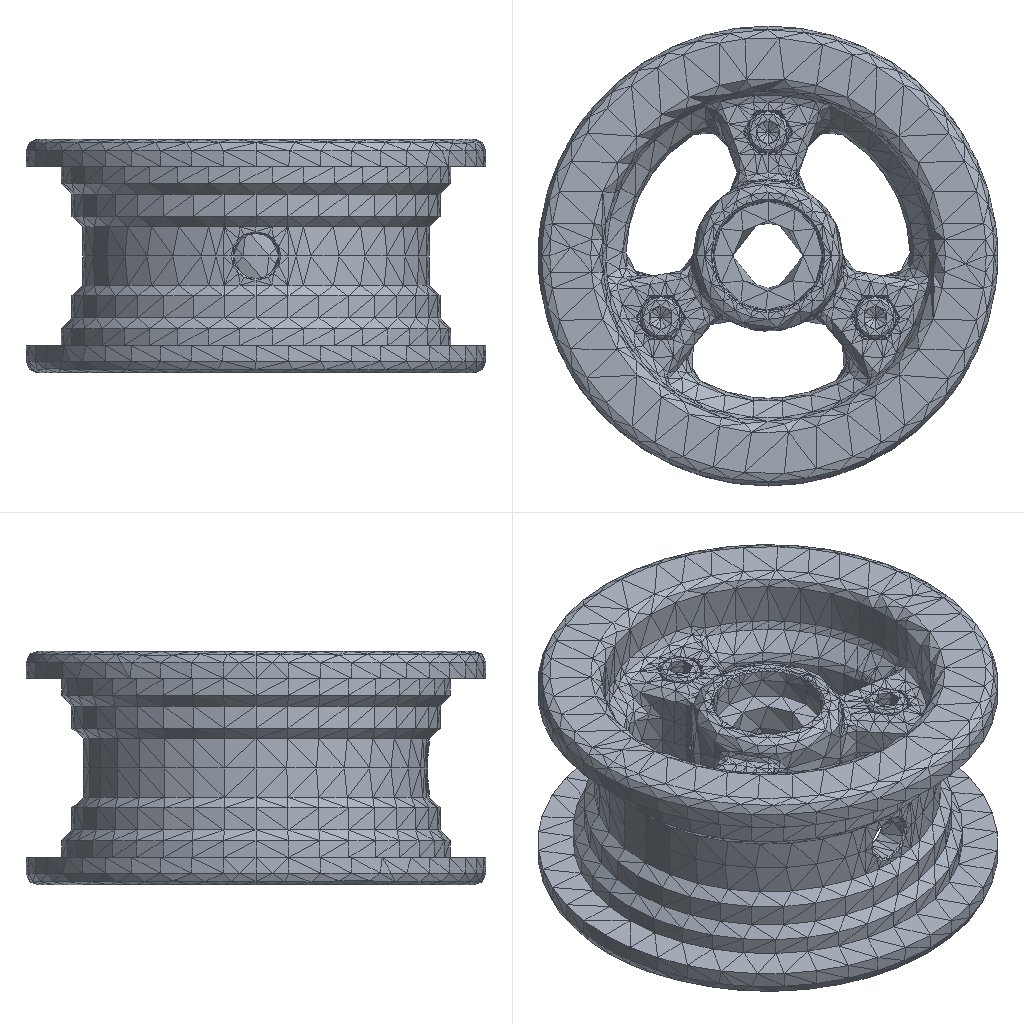Simulation study | ansys workbench
Ansys APDL input file, long lists of numbers shortened:
/batch
/config,noeldb,1     ! force off writing results to database
*get,_wallstrt,active,,time,wall
! ANSYS input file written by Workbench version 2022 R1
! File used for geometry attach:
/title,wbnew--____ (D5)
! ****** Begin Custom Load Command Snippet ******
/COM, ACT Extensions:
/COM,     LSDYNA, 2021.1
/COM,
! ****** End   Custom Load Command Snippet ******
*DIM,_wb_ProjectScratch_dir,string,248
_wb_ProjectScratch_dir(1) = ''
*DIM,_wb_SolverFiles_dir,string,248
_wb_SolverFiles_dir(1) = ''
*DIM,_wb_userfiles_dir,string,248
_wb_userfiles_dir(1) = ''
/com,--- Data in consistent NMM units. See Solving Units in the help system for more information.
/units,MPA
/nopr
/wb,file,start              !  signify a WB generated input file
/prep7
! Turn off shape checking because checks already performed inside WB mesher.
! See help system for more information.
SHPP,OFF,,NOWARN
/nolist
etcon,set             ! allow ANSYS to choose best KEYOP's for 180x elements, resets any applicable keyopt to MAPDL defaults
/com,*********** Nodes for the whole assembly ***********
nblock,3,,38121
(1i9,3e20.9e3)
        1    -5.164900630E+01     4.284439535E+01     3.826096569E+01
! (34655 more lines like these left out)
-1
/com,*********** Nodes for all Remote Points ***********
nblock,3
(1i9,3e20.9e3)
    34657    -5.164900630E+01     1.223253645E+01     3.003884414E+01
-1
/wb,elem,start            !  set before creation of elements
/com,*********** Elements for Body 1 "Wheel Hub|Pah4" ***********
et,1,187
eblock,19,solid,,6596
(19i9)
        1        1        1        1        0        0        0        0       10        0    11937    23119    23893    24445    24099    29033    33173    29038    29035
! (13191 more lines like these left out)
-1
/com,*********** Elements for Body 2 "Wheel Hub|Pah4[2]" ***********
et,2,187
eblock,19,solid,,6596
(19i9)
        2        2        2        2        0        0        0        0       10        0     5341    10933    11707    12259    11913    16847    20987    16852    16849
! (13191 more lines like these left out)
-1
/com,*********** Elements for Body 3 "socket head cap screw_am32323_PreviewCfg|____1" ***********
et,3,187
eblock,19,solid,,671
(19i9)
        3        3        3        3        0        0        0        0       10        0      672     1298     1415     1505     1489     1616     2262     1622     1620
! (1341 more lines like these left out)
-1
/com,*********** Elements for Body 4 "socket head cap screw_am32323_PreviewCfg|____1[2]" ***********
et,4,187
eblock,19,solid,,671
(19i9)
        4        4        4        4        0        0        0        0       10        0     3561     6868     6985     7075     7059     7186     7832     7192     7190
! (1341 more lines like these left out)
-1
/com,*********** Elements for Body 5 "socket head cap screw_am32323_PreviewCfg|____1[3]" ***********
et,5,187
eblock,19,solid,,671
(19i9)
        5        5        5        5        0        0        0        0       10        0        1       12      129      219      203      330      976      336      334
! (1341 more lines like these left out)
-1
/com,*********** Elements for Body 6 "hex nut style 1_am333_PreviewCfg|____1" ***********
et,6,187
eblock,19,solid,,1109
(19i9)
        6        6        6        6        0        0        0        0       10        0     2452     5022     5083     5045     5077     6728     6812     6724     6726
! (2217 more lines like these left out)
-1
/com,*********** Elements for Body 7 "hex nut style 1_am333_PreviewCfg|____1[2]" ***********
et,7,187
eblock,19,solid,,1109
(19i9)
        7        7        7        7        0        0        0        0       10        0     4232     8450     8511     8473     8505    10156    10240    10152    10154
! (2217 more lines like these left out)
-1
/com,*********** Elements for Body 8 "hex nut style 1_am333_PreviewCfg|____1[3]" ***********
et,8,187
eblock,19,solid,,1109
(19i9)
        8        8        8        8        0        0        0        0       10        0     1343     2880     2941     2903     2935     4586     4670     4582     4584
! (2217 more lines like these left out)
-1
/wb,elem,end               !  done creating elements
/com,*********** Send User Defined Coordinate System(s) ***********
csys,0
toffst,273.15,  ! Temperature offset from absolute zero
/com,*********** Set Reference Temperature ***********
tref,22.
/wb,mat,start              !  starting to send materials
/com,*********** Send Materials ***********
Temperature = 'TEMP' ! Temperature
MP,DENS,1,7.85e-09,	! tonne mm^-3
MP,ALPX,1,1.2e-05,	! C^-1
MP,C,1,434000000,	! mm^2 s^-2 C^-1
MP,KXX,1,60.5,	! tonne mm s^-3 C^-1
MP,RSVX,1,0.00017,	! ohm mm
MP,EX,1,200000,	! tonne s^-2 mm^-1
MP,NUXY,1,0.3,
MP,MURX,1,10000,
Temperature = 'TEMP' ! Temperature
MP,DENS,2,7.85e-09,	! tonne mm^-3
MP,ALPX,2,1.2e-05,	! C^-1
MP,C,2,434000000,	! mm^2 s^-2 C^-1
MP,KXX,2,60.5,	! tonne mm s^-3 C^-1
MP,RSVX,2,0.00017,	! ohm mm
MP,EX,2,200000,	! tonne s^-2 mm^-1
MP,NUXY,2,0.3,
MP,MURX,2,10000,
Temperature = 'TEMP' ! Temperature
MP,DENS,3,7.85e-09,	! tonne mm^-3
MP,ALPX,3,1.2e-05,	! C^-1
MP,C,3,434000000,	! mm^2 s^-2 C^-1
MP,KXX,3,60.5,	! tonne mm s^-3 C^-1
MP,RSVX,3,0.00017,	! ohm mm
MP,EX,3,200000,	! tonne s^-2 mm^-1
MP,NUXY,3,0.3,
MP,MURX,3,10000,
Temperature = 'TEMP' ! Temperature
MP,DENS,4,7.85e-09,	! tonne mm^-3
MP,ALPX,4,1.2e-05,	! C^-1
MP,C,4,434000000,	! mm^2 s^-2 C^-1
MP,KXX,4,60.5,	! tonne mm s^-3 C^-1
MP,RSVX,4,0.00017,	! ohm mm
MP,EX,4,200000,	! tonne s^-2 mm^-1
MP,NUXY,4,0.3,
MP,MURX,4,10000,
Temperature = 'TEMP' ! Temperature
MP,DENS,5,7.85e-09,	! tonne mm^-3
MP,ALPX,5,1.2e-05,	! C^-1
MP,C,5,434000000,	! mm^2 s^-2 C^-1
MP,KXX,5,60.5,	! tonne mm s^-3 C^-1
MP,RSVX,5,0.00017,	! ohm mm
MP,EX,5,200000,	! tonne s^-2 mm^-1
MP,NUXY,5,0.3,
MP,MURX,5,10000,
Temperature = 'TEMP' ! Temperature
MP,DENS,6,7.85e-09,	! tonne mm^-3
MP,ALPX,6,1.2e-05,	! C^-1
MP,C,6,434000000,	! mm^2 s^-2 C^-1
MP,KXX,6,60.5,	! tonne mm s^-3 C^-1
MP,RSVX,6,0.00017,	! ohm mm
MP,EX,6,200000,	! tonne s^-2 mm^-1
MP,NUXY,6,0.3,
MP,MURX,6,10000,
Temperature = 'TEMP' ! Temperature
MP,DENS,7,7.85e-09,	! tonne mm^-3
MP,ALPX,7,1.2e-05,	! C^-1
MP,C,7,434000000,	! mm^2 s^-2 C^-1
MP,KXX,7,60.5,	! tonne mm s^-3 C^-1
MP,RSVX,7,0.00017,	! ohm mm
MP,EX,7,200000,	! tonne s^-2 mm^-1
MP,NUXY,7,0.3,
MP,MURX,7,10000,
Temperature = 'TEMP' ! Temperature
MP,DENS,8,7.85e-09,	! tonne mm^-3
MP,ALPX,8,1.2e-05,	! C^-1
MP,C,8,434000000,	! mm^2 s^-2 C^-1
MP,KXX,8,60.5,	! tonne mm s^-3 C^-1
MP,RSVX,8,0.00017,	! ohm mm
MP,EX,8,200000,	! tonne s^-2 mm^-1
MP,NUXY,8,0.3,
MP,MURX,8,10000,
/wb,mat,end                !  done sending materials
!************************* Model Summary ********************
!Wheel Hub|Pah4,	6061,	matid,	1
!Wheel Hub|Pah4[2],	6061,	matid,	2
!socket head cap screw_am32323_PreviewCfg|____1,	6061,	matid,	3
!socket head cap screw_am32323_PreviewCfg|____1[2],	6061,	matid,	4
!socket head cap screw_am32323_PreviewCfg|____1[3],	6061,	matid,	5
!hex nut style 1_am333_PreviewCfg|____1,	6061,	matid,	6
!hex nut style 1_am333_PreviewCfg|____1[2],	6061,	matid,	7
!hex nut style 1_am333_PreviewCfg|____1[3],	6061,	matid,	8
!************************* End Model Summary ********************
! get the diagonal of the bounding box. Needed later for other things
*get,_xmin,node,,mnloc,x
*get,_ymin,node,,mnloc,y
*get,_zmin,node,,mnloc,z
*get,_xmax,node,,mxloc,x
*get,_ymax,node,,mxloc,y
*get,_zmax,node,,mxloc,z
_ASMDIAG=(_xmax-_xmin)*(_xmax-_xmin)+(_ymax-_ymin)*(_ymax-_ymin)+(_zmax-_zmin)*(_zmax-_zmin)
_ASMDIAG=SQRT(_ASMDIAG)
/wb,contact,start          !  starting to send contact
/com,*********** Create Contact "接触区域" ***********
/com,            Real Constant Set For Above Contact Is 10 & 9
*set,tid,10
*set,cid,9
r,tid
r,cid
et,tid,170
et,cid,174
eblock,10,,,292
(15i9)
    27844       10       10       10        0    22495    22497    22499    22499    24605    24622    22499    24606
! (291 more lines like these left out)
-1
eblock,10,,,292
(15i9)
    28136        9        9        9        0    22495    22497    22499    22499    24605    24622    22499    24606
! (291 more lines like these left out)
-1
eblock,10,,,292
(15i9)
    28428        9       10        9        0    10324    10794    11362    11362    12531    15894    11362    12532
! (291 more lines like these left out)
-1
eblock,10,,,292
(15i9)
    28720       10        9       10        0    10324    10794    11362    11362    12531    15894    11362    12532
! (291 more lines like these left out)
-1
keyo,cid,8,2               ! auto create asymmetric contact (from Program Controlled setting)
keyo,cid,10,0              ! adjust contact stiffness each NR iteration (from Program Controlled setting)
keyo,cid,12,5              ! bonded always
keyo,cid,18,1              ! small sliding turned on by application
keyo,cid,2,0               ! augmented Lagrange (from Program Controlled setting)
keyo,cid,4,0               ! on Gauss point (from Program Controlled setting)
keyo,cid,9,1               ! ignore initial gaps/penetration
keyo,cid,7,0               ! No Prediction
rmod,tid,3,10.      ! FKN
rmod,tid,5,0.       ! ICONT
rmod,tid,6,0.       ! PINB
rmod,tid,10,0.      ! CNOF
rmod,tid,12,0.      ! FKT
rmod,tid,36,47      ! WB DSID
rmod,cid,3,10.      ! FKN
rmod,cid,5,0.       ! ICONT
rmod,cid,6,0.       ! PINB
rmod,cid,10,0.      ! CNOF
rmod,cid,12,0.      ! FKT
rmod,cid,36,47      ! WB DSID
/com,*********** Create Contact "接触区域 2" ***********
/com,            Real Constant Set For Above Contact Is 12 & 11
*set,tid,12
*set,cid,11
r,tid
r,cid
et,tid,170
et,cid,174
eblock,10,,,78
(15i9)
    29012       12       12       12        0    22918    22919    23454    23454    27724    27731    23454    27725
! (77 more lines like these left out)
-1
eblock,10,,,78
(15i9)
    29090       11       11       11        0    22918    22919    23454    23454    27724    27731    23454    27725
! (77 more lines like these left out)
-1
eblock,10,,,120
(15i9)
    29168       11       12       11        0     1400     1399     1303     1303     2184     1657     1303     1658
! (119 more lines like these left out)
-1
eblock,10,,,120
(15i9)
    29288       12       11       12        0     1400     1399     1303     1303     2184     1657     1303     1658
! (119 more lines like these left out)
-1
keyo,cid,8,2               ! auto create asymmetric contact (from Program Controlled setting)
keyo,cid,10,0              ! adjust contact stiffness each NR iteration (from Program Controlled setting)
keyo,cid,12,5              ! bonded always
keyo,cid,18,1              ! small sliding turned on by application
keyo,cid,2,0               ! augmented Lagrange (from Program Controlled setting)
keyo,cid,4,0               ! on Gauss point (from Program Controlled setting)
keyo,cid,9,1               ! ignore initial gaps/penetration
keyo,cid,7,0               ! No Prediction
rmod,tid,3,10.      ! FKN
rmod,tid,5,0.       ! ICONT
rmod,tid,6,0.       ! PINB
rmod,tid,10,0.      ! CNOF
rmod,tid,12,0.      ! FKT
rmod,tid,36,50      ! WB DSID
rmod,cid,3,10.      ! FKN
rmod,cid,5,0.       ! ICONT
rmod,cid,6,0.       ! PINB
rmod,cid,10,0.      ! CNOF
rmod,cid,12,0.      ! FKT
rmod,cid,36,50      ! WB DSID
/com,*********** Create Contact "接触区域 3" ***********
/com,            Real Constant Set For Above Contact Is 14 & 13
*set,tid,14
*set,cid,13
r,tid
r,cid
et,tid,170
et,cid,174
eblock,10,,,78
(15i9)
    29408       14       14       14        0    22926    23468    23463    23463    27781    31254    23463    27780
! (77 more lines like these left out)
-1
eblock,10,,,78
(15i9)
    29486       13       13       13        0    22926    23468    23463    23463    27781    31254    23463    27780
! (77 more lines like these left out)
-1
eblock,10,,,120
(15i9)
    29564       13       14       13        0     6970     6969     6873     6873     7754     7227     6873     7228
! (119 more lines like these left out)
-1
eblock,10,,,120
(15i9)
    29684       14       13       14        0     6970     6969     6873     6873     7754     7227     6873     7228
! (119 more lines like these left out)
-1
keyo,cid,8,2               ! auto create asymmetric contact (from Program Controlled setting)
keyo,cid,10,0              ! adjust contact stiffness each NR iteration (from Program Controlled setting)
keyo,cid,12,5              ! bonded always
keyo,cid,18,1              ! small sliding turned on by application
keyo,cid,2,0               ! augmented Lagrange (from Program Controlled setting)
keyo,cid,4,0               ! on Gauss point (from Program Controlled setting)
keyo,cid,9,1               ! ignore initial gaps/penetration
keyo,cid,7,0               ! No Prediction
rmod,tid,3,10.      ! FKN
rmod,tid,5,0.       ! ICONT
rmod,tid,6,0.       ! PINB
rmod,tid,10,0.      ! CNOF
rmod,tid,12,0.      ! FKT
rmod,tid,36,53      ! WB DSID
rmod,cid,3,10.      ! FKN
rmod,cid,5,0.       ! ICONT
rmod,cid,6,0.       ! PINB
rmod,cid,10,0.      ! CNOF
rmod,cid,12,0.      ! FKT
rmod,cid,36,53      ! WB DSID
/com,*********** Create Contact "接触区域 4" ***********
/com,            Real Constant Set For Above Contact Is 16 & 15
*set,tid,16
*set,cid,15
r,tid
r,cid
et,tid,170
et,cid,174
eblock,10,,,96
(15i9)
    29804       16       16       16        0    22908    23705    23140    23140    27661    29200    23140    27658
! (95 more lines like these left out)
-1
eblock,10,,,96
(15i9)
    29900       15       15       15        0    22908    23705    23140    23140    27661    29200    23140    27658
! (95 more lines like these left out)
-1
eblock,10,,,120
(15i9)
    29996       15       16       15        0      114      113       17       17      898      371       17      372
! (119 more lines like these left out)
-1
eblock,10,,,120
(15i9)
    30116       16       15       16        0      114      113       17       17      898      371       17      372
! (119 more lines like these left out)
-1
keyo,cid,8,2               ! auto create asymmetric contact (from Program Controlled setting)
keyo,cid,10,0              ! adjust contact stiffness each NR iteration (from Program Controlled setting)
keyo,cid,12,5              ! bonded always
keyo,cid,18,1              ! small sliding turned on by application
keyo,cid,2,0               ! augmented Lagrange (from Program Controlled setting)
keyo,cid,4,0               ! on Gauss point (from Program Controlled setting)
keyo,cid,9,1               ! ignore initial gaps/penetration
keyo,cid,7,0               ! No Prediction
rmod,tid,3,10.      ! FKN
rmod,tid,5,0.       ! ICONT
rmod,tid,6,0.       ! PINB
rmod,tid,10,0.      ! CNOF
rmod,tid,12,0.      ! FKT
rmod,tid,36,56      ! WB DSID
rmod,cid,3,10.      ! FKN
rmod,cid,5,0.       ! ICONT
rmod,cid,6,0.       ! PINB
rmod,cid,10,0.      ! CNOF
rmod,cid,12,0.      ! FKT
rmod,cid,36,56      ! WB DSID
/com,*********** Create Contact "接触区域 5" ***********
/com,            Real Constant Set For Above Contact Is 18 & 17
*set,tid,18
*set,cid,17
r,tid
r,cid
et,tid,170
et,cid,174
eblock,10,,,12
(15i9)
    30236       18       18       18        0    10732    10733    11268    11268    15538    15545    11268    15539
! (11 more lines like these left out)
-1
eblock,10,,,12
(15i9)
    30248       17       17       17        0    10732    10733    11268    11268    15538    15545    11268    15539
! (11 more lines like these left out)
-1
eblock,10,,,154
(15i9)
    30260       17       18       17        0     4879     4937     4987     4987     6115     6303     4987     6117
! (153 more lines like these left out)
-1
eblock,10,,,154
(15i9)
    30414       18       17       18        0     4879     4937     4987     4987     6115     6303     4987     6117
! (153 more lines like these left out)
-1
keyo,cid,8,2               ! auto create asymmetric contact (from Program Controlled setting)
keyo,cid,10,0              ! adjust contact stiffness each NR iteration (from Program Controlled setting)
keyo,cid,12,5              ! bonded always
keyo,cid,18,1              ! small sliding turned on by application
keyo,cid,2,0               ! augmented Lagrange (from Program Controlled setting)
keyo,cid,4,0               ! on Gauss point (from Program Controlled setting)
keyo,cid,9,1               ! ignore initial gaps/penetration
keyo,cid,7,0               ! No Prediction
rmod,tid,3,10.      ! FKN
rmod,tid,5,0.       ! ICONT
rmod,tid,6,0.       ! PINB
rmod,tid,10,0.      ! CNOF
rmod,tid,12,0.      ! FKT
rmod,tid,36,59      ! WB DSID
rmod,cid,3,10.      ! FKN
rmod,cid,5,0.       ! ICONT
rmod,cid,6,0.       ! PINB
rmod,cid,10,0.      ! CNOF
rmod,cid,12,0.      ! FKT
rmod,cid,36,59      ! WB DSID
/com,*********** Create Contact "接触区域 6" ***********
/com,            Real Constant Set For Above Contact Is 20 & 19
*set,tid,20
*set,cid,19
r,tid
r,cid
et,tid,170
et,cid,174
eblock,10,,,19
(15i9)
    30568       20       20       20        0    10722    11519    10954    10954    15475    17014    10954    15472
! (18 more lines like these left out)
-1
eblock,10,,,19
(15i9)
    30587       19       19       19        0    10722    11519    10954    10954    15475    17014    10954    15472
! (18 more lines like these left out)
-1
eblock,10,,,147
(15i9)
    30606       19       20       19        0     8307     8365     8415     8415     9543     9731     8415     9545
! (146 more lines like these left out)
-1
eblock,10,,,147
(15i9)
    30753       20       19       20        0     8307     8365     8415     8415     9543     9731     8415     9545
! (146 more lines like these left out)
-1
keyo,cid,8,2               ! auto create asymmetric contact (from Program Controlled setting)
keyo,cid,10,0              ! adjust contact stiffness each NR iteration (from Program Controlled setting)
keyo,cid,12,5              ! bonded always
keyo,cid,18,1              ! small sliding turned on by application
keyo,cid,2,0               ! augmented Lagrange (from Program Controlled setting)
keyo,cid,4,0               ! on Gauss point (from Program Controlled setting)
keyo,cid,9,1               ! ignore initial gaps/penetration
keyo,cid,7,0               ! No Prediction
rmod,tid,3,10.      ! FKN
rmod,tid,5,0.       ! ICONT
rmod,tid,6,0.       ! PINB
rmod,tid,10,0.      ! CNOF
rmod,tid,12,0.      ! FKT
rmod,tid,36,62      ! WB DSID
rmod,cid,3,10.      ! FKN
rmod,cid,5,0.       ! ICONT
rmod,cid,6,0.       ! PINB
rmod,cid,10,0.      ! CNOF
rmod,cid,12,0.      ! FKT
rmod,cid,36,62      ! WB DSID
/com,*********** Create Contact "接触区域 7" ***********
/com,            Real Constant Set For Above Contact Is 22 & 21
*set,tid,22
*set,cid,21
r,tid
r,cid
et,tid,170
et,cid,174
eblock,10,,,12
(15i9)
    30900       22       22       22        0    10740    11282    11277    11277    15595    19068    11277    15594
! (11 more lines like these left out)
-1
eblock,10,,,12
(15i9)
    30912       21       21       21        0    10740    11282    11277    11277    15595    19068    11277    15594
! (11 more lines like these left out)
-1
eblock,10,,,154
(15i9)
    30924       21       22       21        0     2737     2795     2845     2845     3973     4161     2845     3975
! (153 more lines like these left out)
-1
eblock,10,,,154
(15i9)
    31078       22       21       22        0     2737     2795     2845     2845     3973     4161     2845     3975
! (153 more lines like these left out)
-1
keyo,cid,8,2               ! auto create asymmetric contact (from Program Controlled setting)
keyo,cid,10,0              ! adjust contact stiffness each NR iteration (from Program Controlled setting)
keyo,cid,12,5              ! bonded always
keyo,cid,18,1              ! small sliding turned on by application
keyo,cid,2,0               ! augmented Lagrange (from Program Controlled setting)
keyo,cid,4,0               ! on Gauss point (from Program Controlled setting)
keyo,cid,9,1               ! ignore initial gaps/penetration
keyo,cid,7,0               ! No Prediction
rmod,tid,3,10.      ! FKN
rmod,tid,5,0.       ! ICONT
rmod,tid,6,0.       ! PINB
rmod,tid,10,0.      ! CNOF
rmod,tid,12,0.      ! FKT
rmod,tid,36,65      ! WB DSID
rmod,cid,3,10.      ! FKN
rmod,cid,5,0.       ! ICONT
rmod,cid,6,0.       ! PINB
rmod,cid,10,0.      ! CNOF
rmod,cid,12,0.      ! FKT
rmod,cid,36,65      ! WB DSID
nsel,all
esel,all
/wb,contact,end            !  done creating contacts
/golist
/wb,load,start             !  starting to send loads
/com,*********** Fixed Supports ***********
CMBLOCK,_FIXEDSU,NODE,      507
(8i10)
        59        60        61        62        63        64        75        76
! (63 more lines like these left out)
cmsel,s,_FIXEDSU
d,all,all
nsel,all
/com,*********** Create Remote Point "内部远程点" ***********
! -------- Remote Point Used by "力矩" --------
*set,tid,24
*set,cid,23
et,cid,174
et,tid,170
keyo,tid,2,1               ! Don't fix the pilot node
keyo,tid,4,111111
keyo,cid,12,5              ! Bonded Contact
keyo,cid,4,1               ! Deformable RBE3 style load
keyo,cid,2,2               ! MPC style contact
eblock,10,,,301
(15i9)
    31232       23       23       23        0    10743    10662    10759    10759    14971    14972    10759    15611
! (300 more lines like these left out)
-1
*set,_npilot,34657
_npilot76=_npilot
type,tid
mat ,cid
real,cid
tshape,pilo
en,31533,_npilot
tshape
/com,*********** Construct Moment Using Remote Attachment ***********
/gst,on,on
fini
*get,_numnode,node,0,count
*get,_numelem,elem,0,count
*get, _MAXELEMNUM, elem, 0, NUM, MAX
*get, _MAXNODENUM, node, 0, NUM, MAX
*get, _MAXELEMTYPE, etyp, 0, NUM, MAX
*get, _MAXREALCONST, real, 0, NUM, MAX
/go
/wb,load,end               !  done creating loads
/com,--- Number of total nodes = %_numnode%
/com,--- Number of contact elements = 3689
/com,--- Number of spring elements = 0
/com,--- Number of bearing elements = 0
/com,--- Number of solid elements = 18532
/com,--- Number of condensed parts = 0
/com,--- Number of total elements = %_numelem%
*get,_wallbsol,active,,time,wall
/com,****************************************************************************
/com,*************************    SOLUTION       ********************************
/com,****************************************************************************
/solu
antype,0                   ! static analysis
_thickRatio=  1     ! Ratio of thick parts in the model
eqsl,pcg,1e-8,,,,,,1
cntr,print,1               ! print out contact info and also make no initial contact an error
dmpoption,emat,no             ! Don't combine emat file for DANSYS
dmpoption,esav,no             ! Don't combine esav file for DANSYS
nldiag,cont,iter           ! print out contact info each equilibrium iteration
rescontrol,,none                 ! Do not keep any restart files
/com,****************************************************
/com,******************* SOLVE FOR LS 1 OF 1 ****************
nsel,s,node,,34657
f,all,mx,0.
f,all,my,0.
f,all,mz,50000.
nsel,all
/nopr
/gopr
nsub,1,1,1
time,1.
outres,erase
outres,all,none
outres,nsol,all,
outres,rsol,all
outres,eangl,all
outres,etmp,all
outres,veng,all
outres,strs,all,
outres,epel,all,
outres,eppl,all,
outres,cont,all,
! *********** WB SOLVE COMMAND ***********
! check interactive state
*get,ANSINTER_,active,,int
*if,ANSINTER_,ne,0,then
/eof
*endif
solve
/com *************** Write FE CONNECTORS *********
CEWRITE,file,ce,,INTE
/com,****************************************************
/com,*************** FINISHED SOLVE FOR LS 1 *************
*get,_wallasol,active,,time,wall
/nopr
*get,_numnode,node,0,count
*get,_numelem,elem,0,count
*get, _MAXELEMNUM, elem, 0, NUM, MAX
*get, _MAXNODENUM, node, 0, NUM, MAX,,,INTERNAL
*get, _MAXELEMTYPE, etyp, 0, NUM, MAX
*get, _MAXREALCONST, real, 0, NUM, MAX
/gopr
*get,_PCGITER,active,,solu,cgiter
/post1
xmlo,ENCODING,ISO-8859-1
xmlo,parm
/xml,parm,xml
fini
/gopr
*get,_walldone,active,,time,wall
_preptime=(_wallbsol-_wallstrt)*3600
_solvtime=(_wallasol-_wallbsol)*3600
_posttime=(_walldone-_wallasol)*3600
_totaltim=(_walldone-_wallstrt)*3600
*get,_dlbratio,active,0,solu,dlbr
*get,_combtime,active,0,solu,comb
*get,_ssmode,active,0,solu,ssmm
*get,_ndofs,active,0,solu,ndof
*get,_sol_end_time,active,0,set,time
*if,_sol_end_time,eq,1.,then
/fclean				!clean distributed files
*endif
/com,--- Total number of nodes = %_numnode%
/com,--- Total number of elements = %_numelem%
/com,--- Element load balance ratio = %_dlbratio%
/com,--- Time to combine distributed files = %_combtime%
/com,--- Sparse memory mode = %_ssmode%
/com,--- Number of DOF = %_ndofs%
/wb,file,end               ! done with WB generated input